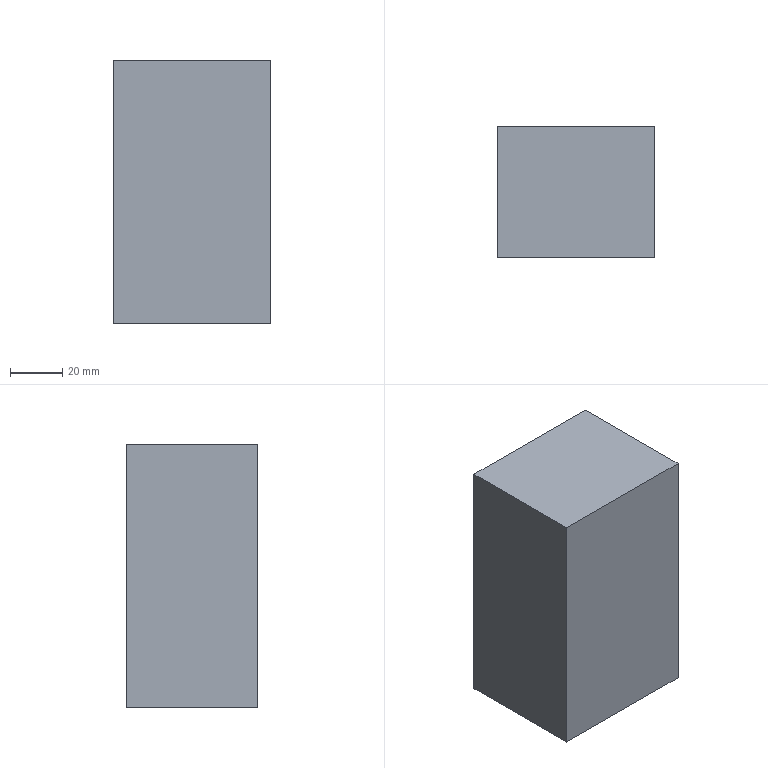Part | SolidWorks | features Extrusion 1 | 1 solid | 6 faces | box 60 x 50 x 100 mm | volume 300000 mm3 | plane 6
STEP:
#1=CARTESIAN_POINT('',(30.,0.,50.));
#2=VERTEX_POINT('',#1);
#3=CARTESIAN_POINT('',(30.,0.,-50.));
#4=VERTEX_POINT('',#3);
#5=CARTESIAN_POINT('',(30.,0.,-50.));
#6=DIRECTION('',(0.,0.,-1.));
#7=VECTOR('',#6,1000.);
#8=LINE('',#5,#7);
#9=EDGE_CURVE('',#2,#4,#8,.T.);
#10=ORIENTED_EDGE('',*,*,#9,.T.);
#11=CARTESIAN_POINT('',(30.,50.,-50.));
#12=VERTEX_POINT('',#11);
#13=CARTESIAN_POINT('',(30.,50.,-50.));
#14=DIRECTION('',(0.,-1.,0.));
#15=VECTOR('',#14,1000.);
#16=LINE('',#13,#15);
#17=EDGE_CURVE('',#12,#4,#16,.T.);
#18=ORIENTED_EDGE('',*,*,#17,.F.);
#19=CARTESIAN_POINT('',(30.,50.,50.));
#20=VERTEX_POINT('',#19);
#21=CARTESIAN_POINT('',(30.,50.,-50.));
#22=DIRECTION('',(0.,0.,-1.));
#23=VECTOR('',#22,1000.);
#24=LINE('',#21,#23);
#25=EDGE_CURVE('',#20,#12,#24,.T.);
#26=ORIENTED_EDGE('',*,*,#25,.F.);
#27=CARTESIAN_POINT('',(30.,50.,50.));
#28=DIRECTION('',(0.,-1.,0.));
#29=VECTOR('',#28,1000.);
#30=LINE('',#27,#29);
#31=EDGE_CURVE('',#20,#2,#30,.T.);
#32=ORIENTED_EDGE('',*,*,#31,.T.);
#33=EDGE_LOOP('',(#10,#18,#26,#32));
#34=FACE_OUTER_BOUND('',#33,.T.);
#35=CARTESIAN_POINT('',(30.,50.,-50.));
#36=DIRECTION('',(-1.,0.,0.));
#37=DIRECTION('',(0.,0.,1.));
#38=AXIS2_PLACEMENT_3D('',#35,#36,#37);
#39=PLANE('',#38);
#40=ADVANCED_FACE('',(#34),#39,.F.);
#41=CARTESIAN_POINT('',(-30.,0.,-50.));
#42=VERTEX_POINT('',#41);
#43=CARTESIAN_POINT('',(-30.,0.,-50.));
#44=DIRECTION('',(-1.,0.,0.));
#45=VECTOR('',#44,1000.);
#46=LINE('',#43,#45);
#47=EDGE_CURVE('',#4,#42,#46,.T.);
#48=ORIENTED_EDGE('',*,*,#47,.T.);
#49=CARTESIAN_POINT('',(-30.,50.,-50.));
#50=VERTEX_POINT('',#49);
#51=CARTESIAN_POINT('',(-30.,50.,-50.));
#52=DIRECTION('',(0.,-1.,0.));
#53=VECTOR('',#52,1000.);
#54=LINE('',#51,#53);
#55=EDGE_CURVE('',#50,#42,#54,.T.);
#56=ORIENTED_EDGE('',*,*,#55,.F.);
#57=CARTESIAN_POINT('',(-30.,50.,-50.));
#58=DIRECTION('',(-1.,0.,0.));
#59=VECTOR('',#58,1000.);
#60=LINE('',#57,#59);
#61=EDGE_CURVE('',#12,#50,#60,.T.);
#62=ORIENTED_EDGE('',*,*,#61,.F.);
#63=ORIENTED_EDGE('',*,*,#17,.T.);
#64=EDGE_LOOP('',(#48,#56,#62,#63));
#65=FACE_OUTER_BOUND('',#64,.T.);
#66=CARTESIAN_POINT('',(-30.,50.,-50.));
#67=DIRECTION('',(0.,0.,1.));
#68=DIRECTION('',(1.,0.,0.));
#69=AXIS2_PLACEMENT_3D('',#66,#67,#68);
#70=PLANE('',#69);
#71=ADVANCED_FACE('',(#65),#70,.F.);
#72=CARTESIAN_POINT('',(-30.,0.,50.));
#73=VERTEX_POINT('',#72);
#74=CARTESIAN_POINT('',(-30.,0.,-50.));
#75=DIRECTION('',(0.,0.,1.));
#76=VECTOR('',#75,1000.);
#77=LINE('',#74,#76);
#78=EDGE_CURVE('',#42,#73,#77,.T.);
#79=ORIENTED_EDGE('',*,*,#78,.T.);
#80=CARTESIAN_POINT('',(-30.,50.,50.));
#81=VERTEX_POINT('',#80);
#82=CARTESIAN_POINT('',(-30.,50.,50.));
#83=DIRECTION('',(0.,-1.,0.));
#84=VECTOR('',#83,1000.);
#85=LINE('',#82,#84);
#86=EDGE_CURVE('',#81,#73,#85,.T.);
#87=ORIENTED_EDGE('',*,*,#86,.F.);
#88=CARTESIAN_POINT('',(-30.,50.,-50.));
#89=DIRECTION('',(0.,0.,1.));
#90=VECTOR('',#89,1000.);
#91=LINE('',#88,#90);
#92=EDGE_CURVE('',#50,#81,#91,.T.);
#93=ORIENTED_EDGE('',*,*,#92,.F.);
#94=ORIENTED_EDGE('',*,*,#55,.T.);
#95=EDGE_LOOP('',(#79,#87,#93,#94));
#96=FACE_OUTER_BOUND('',#95,.T.);
#97=CARTESIAN_POINT('',(-30.,50.,-50.));
#98=DIRECTION('',(1.,0.,0.));
#99=DIRECTION('',(0.,0.,-1.));
#100=AXIS2_PLACEMENT_3D('',#97,#98,#99);
#101=PLANE('',#100);
#102=ADVANCED_FACE('',(#96),#101,.F.);
#103=CARTESIAN_POINT('',(-30.,0.,50.));
#104=DIRECTION('',(1.,0.,0.));
#105=VECTOR('',#104,1000.);
#106=LINE('',#103,#105);
#107=EDGE_CURVE('',#73,#2,#106,.T.);
#108=ORIENTED_EDGE('',*,*,#107,.T.);
#109=ORIENTED_EDGE('',*,*,#31,.F.);
#110=CARTESIAN_POINT('',(-30.,50.,50.));
#111=DIRECTION('',(1.,0.,0.));
#112=VECTOR('',#111,1000.);
#113=LINE('',#110,#112);
#114=EDGE_CURVE('',#81,#20,#113,.T.);
#115=ORIENTED_EDGE('',*,*,#114,.F.);
#116=ORIENTED_EDGE('',*,*,#86,.T.);
#117=EDGE_LOOP('',(#108,#109,#115,#116));
#118=FACE_OUTER_BOUND('',#117,.T.);
#119=CARTESIAN_POINT('',(-30.,50.,50.));
#120=DIRECTION('',(0.,0.,-1.));
#121=DIRECTION('',(-1.,0.,0.));
#122=AXIS2_PLACEMENT_3D('',#119,#120,#121);
#123=PLANE('',#122);
#124=ADVANCED_FACE('',(#118),#123,.F.);
#125=ORIENTED_EDGE('',*,*,#25,.T.);
#126=ORIENTED_EDGE('',*,*,#61,.T.);
#127=ORIENTED_EDGE('',*,*,#92,.T.);
#128=ORIENTED_EDGE('',*,*,#114,.T.);
#129=EDGE_LOOP('',(#125,#126,#127,#128));
#130=FACE_OUTER_BOUND('',#129,.T.);
#131=CARTESIAN_POINT('',(0.,50.,0.));
#132=DIRECTION('',(0.,1.,0.));
#133=DIRECTION('',(0.,0.,1.));
#134=AXIS2_PLACEMENT_3D('',#131,#132,#133);
#135=PLANE('',#134);
#136=ADVANCED_FACE('',(#130),#135,.T.);
#137=ORIENTED_EDGE('',*,*,#9,.F.);
#138=ORIENTED_EDGE('',*,*,#107,.F.);
#139=ORIENTED_EDGE('',*,*,#78,.F.);
#140=ORIENTED_EDGE('',*,*,#47,.F.);
#141=EDGE_LOOP('',(#137,#138,#139,#140));
#142=FACE_OUTER_BOUND('',#141,.T.);
#143=CARTESIAN_POINT('',(0.,0.,0.));
#144=DIRECTION('',(0.,1.,0.));
#145=DIRECTION('',(0.,0.,1.));
#146=AXIS2_PLACEMENT_3D('',#143,#144,#145);
#147=PLANE('',#146);
#148=ADVANCED_FACE('',(#142),#147,.F.);
#149=CLOSED_SHELL('',(#40,#71,#102,#124,#136,#148));
#150=MANIFOLD_SOLID_BREP('',#149);
#151=CARTESIAN_POINT('',(0.,0.,0.));
#152=DIRECTION('',(0.,0.,1.));
#153=DIRECTION('',(1.,0.,0.));
#154=AXIS2_PLACEMENT_3D('',#151,#152,#153);
#155=(LENGTH_UNIT()NAMED_UNIT(*)SI_UNIT(.MILLI.,.METRE.));
#156=UNCERTAINTY_MEASURE_WITH_UNIT(LENGTH_MEASURE(0.00001),#155,'','');
#157=(NAMED_UNIT(*)PLANE_ANGLE_UNIT()SI_UNIT($,.RADIAN.));
#158=(NAMED_UNIT(*)SI_UNIT($,.STERADIAN.)SOLID_ANGLE_UNIT());
#159=(GEOMETRIC_REPRESENTATION_CONTEXT(3)GLOBAL_UNCERTAINTY_ASSIGNED_CONTEXT((#156))GLOBAL_UNIT_ASSIGNED_CONTEXT((#155,#157,#158))REPRESENTATION_CONTEXT('',''));
#160=ADVANCED_BREP_SHAPE_REPRESENTATION('',(#150,#154),#159);